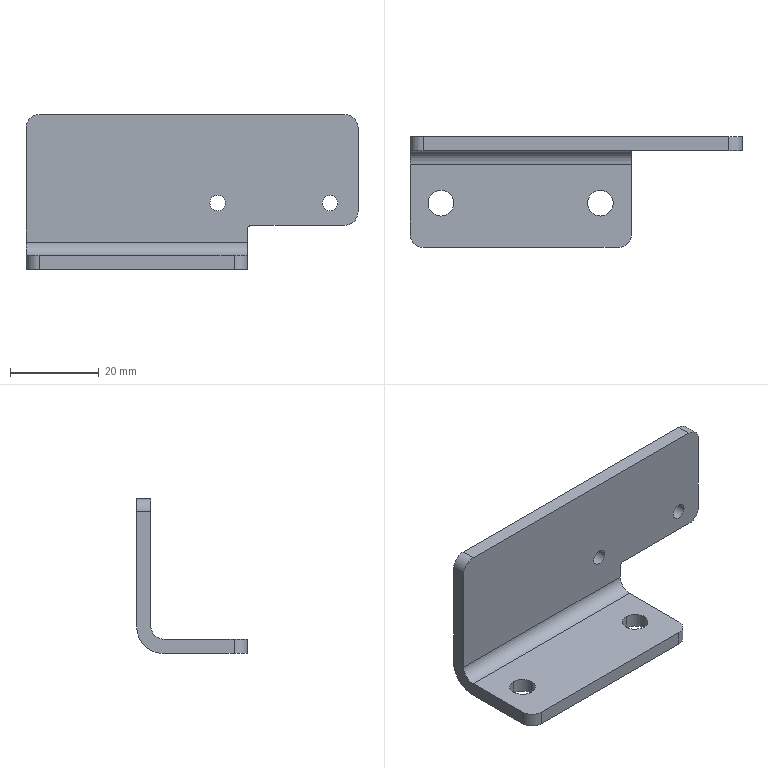Part | STEP file | J014-EBZ05-02-06-Part-1 | 1 solid | 26 faces | box 75 x 25 x 35 mm | volume 10537 mm3 | cylinder 16 | plane 10 | commonest cylinder face diameters 6 x6 3.5 x4 5.8 x4 2 x1 12 x1
STEP:
#1=CARTESIAN_POINT('',(41.55,0.,15.));
#2=VERTEX_POINT('',#1);
#3=CARTESIAN_POINT('',(45.05,0.,15.));
#4=VERTEX_POINT('',#3);
#5=CARTESIAN_POINT('',(43.3,0.,15.));
#6=DIRECTION('',(0.,-1.,0.));
#7=DIRECTION('',(1.,0.,0.));
#8=AXIS2_PLACEMENT_3D('',#5,#6,#7);
#9=CIRCLE('',#8,1.75);
#10=EDGE_CURVE('',#2,#4,#9,.T.);
#11=ORIENTED_EDGE('',*,*,#10,.F.);
#12=CARTESIAN_POINT('',(41.55,-3.2,15.));
#13=VERTEX_POINT('',#12);
#14=CARTESIAN_POINT('',(41.55,0.,15.));
#15=DIRECTION('',(0.,-1.,0.));
#16=VECTOR('',#15,1000.);
#17=LINE('',#14,#16);
#18=EDGE_CURVE('',#2,#13,#17,.T.);
#19=ORIENTED_EDGE('',*,*,#18,.T.);
#20=CARTESIAN_POINT('',(45.05,-3.2,15.));
#21=VERTEX_POINT('',#20);
#22=CARTESIAN_POINT('',(43.3,-3.2,15.));
#23=DIRECTION('',(0.,1.,0.));
#24=DIRECTION('',(-1.,0.,0.));
#25=AXIS2_PLACEMENT_3D('',#22,#23,#24);
#26=CIRCLE('',#25,1.75);
#27=EDGE_CURVE('',#21,#13,#26,.T.);
#28=ORIENTED_EDGE('',*,*,#27,.F.);
#29=CARTESIAN_POINT('',(45.05,0.,15.));
#30=DIRECTION('',(0.,-1.,0.));
#31=VECTOR('',#30,1000.);
#32=LINE('',#29,#31);
#33=EDGE_CURVE('',#4,#21,#32,.T.);
#34=ORIENTED_EDGE('',*,*,#33,.F.);
#35=EDGE_LOOP('',(#11,#19,#28,#34));
#36=FACE_OUTER_BOUND('',#35,.T.);
#37=CARTESIAN_POINT('',(43.3,0.,15.));
#38=DIRECTION('',(0.,-1.,0.));
#39=DIRECTION('',(1.,0.,0.));
#40=AXIS2_PLACEMENT_3D('',#37,#38,#39);
#41=CYLINDRICAL_SURFACE('',#40,1.75);
#42=ADVANCED_FACE('',(#36),#41,.F.);
#43=CARTESIAN_POINT('',(66.95,0.,15.));
#44=VERTEX_POINT('',#43);
#45=CARTESIAN_POINT('',(70.45,0.,15.));
#46=VERTEX_POINT('',#45);
#47=CARTESIAN_POINT('',(68.7,0.,15.));
#48=DIRECTION('',(0.,-1.,0.));
#49=DIRECTION('',(1.,0.,0.));
#50=AXIS2_PLACEMENT_3D('',#47,#48,#49);
#51=CIRCLE('',#50,1.75);
#52=EDGE_CURVE('',#44,#46,#51,.T.);
#53=ORIENTED_EDGE('',*,*,#52,.F.);
#54=CARTESIAN_POINT('',(66.95,-3.2,15.));
#55=VERTEX_POINT('',#54);
#56=CARTESIAN_POINT('',(66.95,0.,15.));
#57=DIRECTION('',(0.,-1.,0.));
#58=VECTOR('',#57,1000.);
#59=LINE('',#56,#58);
#60=EDGE_CURVE('',#44,#55,#59,.T.);
#61=ORIENTED_EDGE('',*,*,#60,.T.);
#62=CARTESIAN_POINT('',(70.45,-3.2,15.));
#63=VERTEX_POINT('',#62);
#64=CARTESIAN_POINT('',(68.7,-3.2,15.));
#65=DIRECTION('',(0.,1.,0.));
#66=DIRECTION('',(-1.,0.,0.));
#67=AXIS2_PLACEMENT_3D('',#64,#65,#66);
#68=CIRCLE('',#67,1.75);
#69=EDGE_CURVE('',#63,#55,#68,.T.);
#70=ORIENTED_EDGE('',*,*,#69,.F.);
#71=CARTESIAN_POINT('',(70.45,0.,15.));
#72=DIRECTION('',(0.,-1.,0.));
#73=VECTOR('',#72,1000.);
#74=LINE('',#71,#73);
#75=EDGE_CURVE('',#46,#63,#74,.T.);
#76=ORIENTED_EDGE('',*,*,#75,.F.);
#77=EDGE_LOOP('',(#53,#61,#70,#76));
#78=FACE_OUTER_BOUND('',#77,.T.);
#79=CARTESIAN_POINT('',(68.7,0.,15.));
#80=DIRECTION('',(0.,-1.,0.));
#81=DIRECTION('',(1.,0.,0.));
#82=AXIS2_PLACEMENT_3D('',#79,#80,#81);
#83=CYLINDRICAL_SURFACE('',#82,1.75);
#84=ADVANCED_FACE('',(#78),#83,.F.);
#85=CARTESIAN_POINT('',(7.,-17.9,3.2));
#86=VERTEX_POINT('',#85);
#87=CARTESIAN_POINT('',(7.,-12.1,3.2));
#88=VERTEX_POINT('',#87);
#89=CARTESIAN_POINT('',(7.,-15.,3.2));
#90=DIRECTION('',(0.,0.,-1.));
#91=DIRECTION('',(0.,1.,0.));
#92=AXIS2_PLACEMENT_3D('',#89,#90,#91);
#93=CIRCLE('',#92,2.9);
#94=EDGE_CURVE('',#86,#88,#93,.T.);
#95=ORIENTED_EDGE('',*,*,#94,.F.);
#96=CARTESIAN_POINT('',(7.,-17.9,0.));
#97=VERTEX_POINT('',#96);
#98=CARTESIAN_POINT('',(7.,-17.9,3.2));
#99=DIRECTION('',(0.,0.,-1.));
#100=VECTOR('',#99,1000.);
#101=LINE('',#98,#100);
#102=EDGE_CURVE('',#86,#97,#101,.T.);
#103=ORIENTED_EDGE('',*,*,#102,.T.);
#104=CARTESIAN_POINT('',(7.,-12.1,0.));
#105=VERTEX_POINT('',#104);
#106=CARTESIAN_POINT('',(7.,-15.,0.));
#107=DIRECTION('',(0.,0.,-1.));
#108=DIRECTION('',(0.,1.,0.));
#109=AXIS2_PLACEMENT_3D('',#106,#107,#108);
#110=CIRCLE('',#109,2.9);
#111=EDGE_CURVE('',#97,#105,#110,.T.);
#112=ORIENTED_EDGE('',*,*,#111,.T.);
#113=CARTESIAN_POINT('',(7.,-12.1,3.2));
#114=DIRECTION('',(0.,0.,-1.));
#115=VECTOR('',#114,1000.);
#116=LINE('',#113,#115);
#117=EDGE_CURVE('',#88,#105,#116,.T.);
#118=ORIENTED_EDGE('',*,*,#117,.F.);
#119=EDGE_LOOP('',(#95,#103,#112,#118));
#120=FACE_OUTER_BOUND('',#119,.T.);
#121=CARTESIAN_POINT('',(7.,-15.,3.2));
#122=DIRECTION('',(0.,0.,-1.));
#123=DIRECTION('',(0.,1.,0.));
#124=AXIS2_PLACEMENT_3D('',#121,#122,#123);
#125=CYLINDRICAL_SURFACE('',#124,2.9);
#126=ADVANCED_FACE('',(#120),#125,.F.);
#127=CARTESIAN_POINT('',(43.,-17.9,3.2));
#128=VERTEX_POINT('',#127);
#129=CARTESIAN_POINT('',(43.,-12.1,3.2));
#130=VERTEX_POINT('',#129);
#131=CARTESIAN_POINT('',(43.,-15.,3.2));
#132=DIRECTION('',(0.,0.,-1.));
#133=DIRECTION('',(0.,1.,0.));
#134=AXIS2_PLACEMENT_3D('',#131,#132,#133);
#135=CIRCLE('',#134,2.9);
#136=EDGE_CURVE('',#128,#130,#135,.T.);
#137=ORIENTED_EDGE('',*,*,#136,.F.);
#138=CARTESIAN_POINT('',(43.,-17.9,0.));
#139=VERTEX_POINT('',#138);
#140=CARTESIAN_POINT('',(43.,-17.9,3.2));
#141=DIRECTION('',(0.,0.,-1.));
#142=VECTOR('',#141,1000.);
#143=LINE('',#140,#142);
#144=EDGE_CURVE('',#128,#139,#143,.T.);
#145=ORIENTED_EDGE('',*,*,#144,.T.);
#146=CARTESIAN_POINT('',(43.,-12.1,0.));
#147=VERTEX_POINT('',#146);
#148=CARTESIAN_POINT('',(43.,-15.,0.));
#149=DIRECTION('',(0.,0.,-1.));
#150=DIRECTION('',(0.,1.,0.));
#151=AXIS2_PLACEMENT_3D('',#148,#149,#150);
#152=CIRCLE('',#151,2.9);
#153=EDGE_CURVE('',#139,#147,#152,.T.);
#154=ORIENTED_EDGE('',*,*,#153,.T.);
#155=CARTESIAN_POINT('',(43.,-12.1,3.2));
#156=DIRECTION('',(0.,0.,-1.));
#157=VECTOR('',#156,1000.);
#158=LINE('',#155,#157);
#159=EDGE_CURVE('',#130,#147,#158,.T.);
#160=ORIENTED_EDGE('',*,*,#159,.F.);
#161=EDGE_LOOP('',(#137,#145,#154,#160));
#162=FACE_OUTER_BOUND('',#161,.T.);
#163=CARTESIAN_POINT('',(43.,-15.,3.2));
#164=DIRECTION('',(0.,0.,-1.));
#165=DIRECTION('',(0.,1.,0.));
#166=AXIS2_PLACEMENT_3D('',#163,#164,#165);
#167=CYLINDRICAL_SURFACE('',#166,2.9);
#168=ADVANCED_FACE('',(#162),#167,.F.);
#169=CARTESIAN_POINT('',(7.,-15.,3.2));
#170=DIRECTION('',(0.,0.,-1.));
#171=DIRECTION('',(0.,1.,0.));
#172=AXIS2_PLACEMENT_3D('',#169,#170,#171);
#173=CIRCLE('',#172,2.9);
#174=EDGE_CURVE('',#88,#86,#173,.T.);
#175=ORIENTED_EDGE('',*,*,#174,.T.);
#176=ORIENTED_EDGE('',*,*,#94,.T.);
#177=EDGE_LOOP('',(#175,#176));
#178=FACE_BOUND('',#177,.T.);
#179=CARTESIAN_POINT('',(43.,-15.,3.2));
#180=DIRECTION('',(0.,0.,-1.));
#181=DIRECTION('',(0.,1.,0.));
#182=AXIS2_PLACEMENT_3D('',#179,#180,#181);
#183=CIRCLE('',#182,2.9);
#184=EDGE_CURVE('',#130,#128,#183,.T.);
#185=ORIENTED_EDGE('',*,*,#184,.T.);
#186=ORIENTED_EDGE('',*,*,#136,.T.);
#187=EDGE_LOOP('',(#185,#186));
#188=FACE_BOUND('',#187,.T.);
#189=CARTESIAN_POINT('',(47.,-25.,3.2));
#190=VERTEX_POINT('',#189);
#191=CARTESIAN_POINT('',(3.,-25.,3.2));
#192=VERTEX_POINT('',#191);
#193=CARTESIAN_POINT('',(25.,-25.,3.2));
#194=DIRECTION('',(-1.,0.,0.));
#195=VECTOR('',#194,1000.);
#196=LINE('',#193,#195);
#197=EDGE_CURVE('',#190,#192,#196,.T.);
#198=ORIENTED_EDGE('',*,*,#197,.F.);
#199=CARTESIAN_POINT('',(50.,-22.,3.2));
#200=VERTEX_POINT('',#199);
#201=CARTESIAN_POINT('',(47.,-22.,3.2));
#202=DIRECTION('',(0.,0.,1.));
#203=DIRECTION('',(0.,-1.,0.));
#204=AXIS2_PLACEMENT_3D('',#201,#202,#203);
#205=CIRCLE('',#204,3.);
#206=EDGE_CURVE('',#190,#200,#205,.T.);
#207=ORIENTED_EDGE('',*,*,#206,.T.);
#208=CARTESIAN_POINT('',(50.,-6.2,3.2));
#209=VERTEX_POINT('',#208);
#210=CARTESIAN_POINT('',(50.,-12.5,3.2));
#211=DIRECTION('',(0.,-1.,0.));
#212=VECTOR('',#211,1000.);
#213=LINE('',#210,#212);
#214=EDGE_CURVE('',#209,#200,#213,.T.);
#215=ORIENTED_EDGE('',*,*,#214,.F.);
#216=CARTESIAN_POINT('',(0.,-6.2,3.2));
#217=VERTEX_POINT('',#216);
#218=CARTESIAN_POINT('',(0.,-6.2,3.2));
#219=DIRECTION('',(-1.,0.,0.));
#220=VECTOR('',#219,1000.);
#221=LINE('',#218,#220);
#222=EDGE_CURVE('',#209,#217,#221,.T.);
#223=ORIENTED_EDGE('',*,*,#222,.T.);
#224=CARTESIAN_POINT('',(0.,-22.,3.2));
#225=VERTEX_POINT('',#224);
#226=CARTESIAN_POINT('',(0.,-12.5,3.2));
#227=DIRECTION('',(0.,1.,0.));
#228=VECTOR('',#227,1000.);
#229=LINE('',#226,#228);
#230=EDGE_CURVE('',#225,#217,#229,.T.);
#231=ORIENTED_EDGE('',*,*,#230,.F.);
#232=CARTESIAN_POINT('',(3.,-22.,3.2));
#233=DIRECTION('',(0.,0.,1.));
#234=DIRECTION('',(0.,-1.,0.));
#235=AXIS2_PLACEMENT_3D('',#232,#233,#234);
#236=CIRCLE('',#235,3.);
#237=EDGE_CURVE('',#225,#192,#236,.T.);
#238=ORIENTED_EDGE('',*,*,#237,.T.);
#239=EDGE_LOOP('',(#198,#207,#215,#223,#231,#238));
#240=FACE_OUTER_BOUND('',#239,.T.);
#241=CARTESIAN_POINT('',(25.,-12.5,3.2));
#242=DIRECTION('',(0.,0.,1.));
#243=DIRECTION('',(0.,-1.,0.));
#244=AXIS2_PLACEMENT_3D('',#241,#242,#243);
#245=PLANE('',#244);
#246=ADVANCED_FACE('',(#178,#188,#240),#245,.T.);
#247=CARTESIAN_POINT('',(0.,-3.2,6.2));
#248=VERTEX_POINT('',#247);
#249=CARTESIAN_POINT('',(0.,-3.2,32.));
#250=VERTEX_POINT('',#249);
#251=CARTESIAN_POINT('',(0.,-3.2,3.2));
#252=DIRECTION('',(0.,0.,1.));
#253=VECTOR('',#252,1000.);
#254=LINE('',#251,#253);
#255=EDGE_CURVE('',#248,#250,#254,.T.);
#256=ORIENTED_EDGE('',*,*,#255,.T.);
#257=CARTESIAN_POINT('',(0.,0.,32.));
#258=VERTEX_POINT('',#257);
#259=CARTESIAN_POINT('',(0.,-12.5,32.));
#260=DIRECTION('',(0.,1.,0.));
#261=VECTOR('',#260,1000.);
#262=LINE('',#259,#261);
#263=EDGE_CURVE('',#250,#258,#262,.T.);
#264=ORIENTED_EDGE('',*,*,#263,.T.);
#265=CARTESIAN_POINT('',(0.,0.,6.));
#266=VERTEX_POINT('',#265);
#267=CARTESIAN_POINT('',(0.,0.,0.));
#268=DIRECTION('',(0.,0.,1.));
#269=VECTOR('',#268,1000.);
#270=LINE('',#267,#269);
#271=EDGE_CURVE('',#266,#258,#270,.T.);
#272=ORIENTED_EDGE('',*,*,#271,.F.);
#273=CARTESIAN_POINT('',(0.,-6.,0.));
#274=VERTEX_POINT('',#273);
#275=CARTESIAN_POINT('',(0.,-6.,6.));
#276=DIRECTION('',(-1.,0.,0.));
#277=DIRECTION('',(0.,0.,-1.));
#278=AXIS2_PLACEMENT_3D('',#275,#276,#277);
#279=CIRCLE('',#278,6.);
#280=EDGE_CURVE('',#266,#274,#279,.T.);
#281=ORIENTED_EDGE('',*,*,#280,.T.);
#282=CARTESIAN_POINT('',(0.,-22.,0.));
#283=VERTEX_POINT('',#282);
#284=CARTESIAN_POINT('',(0.,-12.5,0.));
#285=DIRECTION('',(0.,-1.,0.));
#286=VECTOR('',#285,1000.);
#287=LINE('',#284,#286);
#288=EDGE_CURVE('',#274,#283,#287,.T.);
#289=ORIENTED_EDGE('',*,*,#288,.T.);
#290=CARTESIAN_POINT('',(0.,-22.,0.));
#291=DIRECTION('',(0.,0.,1.));
#292=VECTOR('',#291,1000.);
#293=LINE('',#290,#292);
#294=EDGE_CURVE('',#283,#225,#293,.T.);
#295=ORIENTED_EDGE('',*,*,#294,.T.);
#296=ORIENTED_EDGE('',*,*,#230,.T.);
#297=CARTESIAN_POINT('',(0.,-6.2,6.2));
#298=DIRECTION('',(1.,0.,0.));
#299=DIRECTION('',(0.,0.,-1.));
#300=AXIS2_PLACEMENT_3D('',#297,#298,#299);
#301=CIRCLE('',#300,3.);
#302=EDGE_CURVE('',#217,#248,#301,.T.);
#303=ORIENTED_EDGE('',*,*,#302,.T.);
#304=EDGE_LOOP('',(#256,#264,#272,#281,#289,#295,#296,#303));
#305=FACE_OUTER_BOUND('',#304,.T.);
#306=CARTESIAN_POINT('',(0.,-12.5,0.));
#307=DIRECTION('',(-1.,0.,0.));
#308=DIRECTION('',(0.,0.,-1.));
#309=AXIS2_PLACEMENT_3D('',#306,#307,#308);
#310=PLANE('',#309);
#311=ADVANCED_FACE('',(#305),#310,.T.);
#312=CARTESIAN_POINT('',(43.3,0.,15.));
#313=DIRECTION('',(0.,-1.,0.));
#314=DIRECTION('',(1.,0.,0.));
#315=AXIS2_PLACEMENT_3D('',#312,#313,#314);
#316=CIRCLE('',#315,1.75);
#317=EDGE_CURVE('',#4,#2,#316,.T.);
#318=ORIENTED_EDGE('',*,*,#317,.T.);
#319=ORIENTED_EDGE('',*,*,#10,.T.);
#320=EDGE_LOOP('',(#318,#319));
#321=FACE_BOUND('',#320,.T.);
#322=CARTESIAN_POINT('',(68.7,0.,15.));
#323=DIRECTION('',(0.,-1.,0.));
#324=DIRECTION('',(1.,0.,0.));
#325=AXIS2_PLACEMENT_3D('',#322,#323,#324);
#326=CIRCLE('',#325,1.75);
#327=EDGE_CURVE('',#46,#44,#326,.T.);
#328=ORIENTED_EDGE('',*,*,#327,.T.);
#329=ORIENTED_EDGE('',*,*,#52,.T.);
#330=EDGE_LOOP('',(#328,#329));
#331=FACE_BOUND('',#330,.T.);
#332=CARTESIAN_POINT('',(75.,0.,13.));
#333=VERTEX_POINT('',#332);
#334=CARTESIAN_POINT('',(75.,0.,32.));
#335=VERTEX_POINT('',#334);
#336=CARTESIAN_POINT('',(75.,0.,22.5));
#337=DIRECTION('',(0.,0.,1.));
#338=VECTOR('',#337,1000.);
#339=LINE('',#336,#338);
#340=EDGE_CURVE('',#333,#335,#339,.T.);
#341=ORIENTED_EDGE('',*,*,#340,.F.);
#342=CARTESIAN_POINT('',(72.,0.,10.));
#343=VERTEX_POINT('',#342);
#344=CARTESIAN_POINT('',(72.,0.,13.));
#345=DIRECTION('',(0.,1.,0.));
#346=DIRECTION('',(0.,0.,1.));
#347=AXIS2_PLACEMENT_3D('',#344,#345,#346);
#348=CIRCLE('',#347,3.);
#349=EDGE_CURVE('',#333,#343,#348,.T.);
#350=ORIENTED_EDGE('',*,*,#349,.T.);
#351=CARTESIAN_POINT('',(51.,0.,10.));
#352=VERTEX_POINT('',#351);
#353=CARTESIAN_POINT('',(62.5,0.,10.));
#354=DIRECTION('',(1.,0.,0.));
#355=VECTOR('',#354,1000.);
#356=LINE('',#353,#355);
#357=EDGE_CURVE('',#352,#343,#356,.T.);
#358=ORIENTED_EDGE('',*,*,#357,.F.);
#359=CARTESIAN_POINT('',(50.,0.,9.));
#360=VERTEX_POINT('',#359);
#361=CARTESIAN_POINT('',(51.,0.,9.));
#362=DIRECTION('',(0.,-1.,0.));
#363=DIRECTION('',(0.,0.,1.));
#364=AXIS2_PLACEMENT_3D('',#361,#362,#363);
#365=CIRCLE('',#364,1.);
#366=EDGE_CURVE('',#352,#360,#365,.T.);
#367=ORIENTED_EDGE('',*,*,#366,.T.);
#368=CARTESIAN_POINT('',(50.,0.,6.));
#369=VERTEX_POINT('',#368);
#370=CARTESIAN_POINT('',(50.,0.,0.));
#371=DIRECTION('',(0.,0.,1.));
#372=VECTOR('',#371,1000.);
#373=LINE('',#370,#372);
#374=EDGE_CURVE('',#369,#360,#373,.T.);
#375=ORIENTED_EDGE('',*,*,#374,.F.);
#376=CARTESIAN_POINT('',(25.,0.,6.));
#377=DIRECTION('',(-1.,0.,0.));
#378=VECTOR('',#377,1000.);
#379=LINE('',#376,#378);
#380=EDGE_CURVE('',#369,#266,#379,.T.);
#381=ORIENTED_EDGE('',*,*,#380,.T.);
#382=ORIENTED_EDGE('',*,*,#271,.T.);
#383=CARTESIAN_POINT('',(3.,0.,35.));
#384=VERTEX_POINT('',#383);
#385=CARTESIAN_POINT('',(3.,0.,32.));
#386=DIRECTION('',(0.,1.,0.));
#387=DIRECTION('',(0.,0.,1.));
#388=AXIS2_PLACEMENT_3D('',#385,#386,#387);
#389=CIRCLE('',#388,3.);
#390=EDGE_CURVE('',#258,#384,#389,.T.);
#391=ORIENTED_EDGE('',*,*,#390,.T.);
#392=CARTESIAN_POINT('',(72.,0.,35.));
#393=VERTEX_POINT('',#392);
#394=CARTESIAN_POINT('',(25.,0.,35.));
#395=DIRECTION('',(1.,0.,0.));
#396=VECTOR('',#395,1000.);
#397=LINE('',#394,#396);
#398=EDGE_CURVE('',#384,#393,#397,.T.);
#399=ORIENTED_EDGE('',*,*,#398,.T.);
#400=CARTESIAN_POINT('',(72.,0.,32.));
#401=DIRECTION('',(0.,1.,0.));
#402=DIRECTION('',(0.,0.,1.));
#403=AXIS2_PLACEMENT_3D('',#400,#401,#402);
#404=CIRCLE('',#403,3.);
#405=EDGE_CURVE('',#393,#335,#404,.T.);
#406=ORIENTED_EDGE('',*,*,#405,.T.);
#407=EDGE_LOOP('',(#341,#350,#358,#367,#375,#381,#382,#391,#399,#406));
#408=FACE_OUTER_BOUND('',#407,.T.);
#409=CARTESIAN_POINT('',(25.,0.,0.));
#410=DIRECTION('',(0.,1.,0.));
#411=DIRECTION('',(0.,0.,1.));
#412=AXIS2_PLACEMENT_3D('',#409,#410,#411);
#413=PLANE('',#412);
#414=ADVANCED_FACE('',(#321,#331,#408),#413,.T.);
#415=ORIENTED_EDGE('',*,*,#374,.T.);
#416=CARTESIAN_POINT('',(50.,-3.2,9.));
#417=VERTEX_POINT('',#416);
#418=CARTESIAN_POINT('',(50.,-3.2,9.));
#419=DIRECTION('',(0.,-1.,0.));
#420=VECTOR('',#419,1000.);
#421=LINE('',#418,#420);
#422=EDGE_CURVE('',#360,#417,#421,.T.);
#423=ORIENTED_EDGE('',*,*,#422,.T.);
#424=CARTESIAN_POINT('',(50.,-3.2,6.2));
#425=VERTEX_POINT('',#424);
#426=CARTESIAN_POINT('',(50.,-3.2,3.2));
#427=DIRECTION('',(0.,0.,1.));
#428=VECTOR('',#427,1000.);
#429=LINE('',#426,#428);
#430=EDGE_CURVE('',#425,#417,#429,.T.);
#431=ORIENTED_EDGE('',*,*,#430,.F.);
#432=CARTESIAN_POINT('',(50.,-6.2,6.2));
#433=DIRECTION('',(-1.,0.,0.));
#434=DIRECTION('',(0.,0.,1.));
#435=AXIS2_PLACEMENT_3D('',#432,#433,#434);
#436=CIRCLE('',#435,3.);
#437=EDGE_CURVE('',#425,#209,#436,.T.);
#438=ORIENTED_EDGE('',*,*,#437,.T.);
#439=ORIENTED_EDGE('',*,*,#214,.T.);
#440=CARTESIAN_POINT('',(50.,-22.,0.));
#441=VERTEX_POINT('',#440);
#442=CARTESIAN_POINT('',(50.,-22.,0.));
#443=DIRECTION('',(0.,0.,-1.));
#444=VECTOR('',#443,1000.);
#445=LINE('',#442,#444);
#446=EDGE_CURVE('',#200,#441,#445,.T.);
#447=ORIENTED_EDGE('',*,*,#446,.T.);
#448=CARTESIAN_POINT('',(50.,-6.,0.));
#449=VERTEX_POINT('',#448);
#450=CARTESIAN_POINT('',(50.,-12.5,0.));
#451=DIRECTION('',(0.,1.,0.));
#452=VECTOR('',#451,1000.);
#453=LINE('',#450,#452);
#454=EDGE_CURVE('',#441,#449,#453,.T.);
#455=ORIENTED_EDGE('',*,*,#454,.T.);
#456=CARTESIAN_POINT('',(50.,-6.,6.));
#457=DIRECTION('',(1.,0.,0.));
#458=DIRECTION('',(0.,0.,1.));
#459=AXIS2_PLACEMENT_3D('',#456,#457,#458);
#460=CIRCLE('',#459,6.);
#461=EDGE_CURVE('',#449,#369,#460,.T.);
#462=ORIENTED_EDGE('',*,*,#461,.T.);
#463=EDGE_LOOP('',(#415,#423,#431,#438,#439,#447,#455,#462));
#464=FACE_OUTER_BOUND('',#463,.T.);
#465=CARTESIAN_POINT('',(50.,-12.5,0.));
#466=DIRECTION('',(1.,0.,0.));
#467=DIRECTION('',(0.,0.,1.));
#468=AXIS2_PLACEMENT_3D('',#465,#466,#467);
#469=PLANE('',#468);
#470=ADVANCED_FACE('',(#464),#469,.T.);
#471=CARTESIAN_POINT('',(7.,-15.,0.));
#472=DIRECTION('',(0.,0.,-1.));
#473=DIRECTION('',(0.,1.,0.));
#474=AXIS2_PLACEMENT_3D('',#471,#472,#473);
#475=CIRCLE('',#474,2.9);
#476=EDGE_CURVE('',#105,#97,#475,.T.);
#477=ORIENTED_EDGE('',*,*,#476,.F.);
#478=ORIENTED_EDGE('',*,*,#111,.F.);
#479=EDGE_LOOP('',(#477,#478));
#480=FACE_BOUND('',#479,.T.);
#481=CARTESIAN_POINT('',(43.,-15.,0.));
#482=DIRECTION('',(0.,0.,-1.));
#483=DIRECTION('',(0.,1.,0.));
#484=AXIS2_PLACEMENT_3D('',#481,#482,#483);
#485=CIRCLE('',#484,2.9);
#486=EDGE_CURVE('',#147,#139,#485,.T.);
#487=ORIENTED_EDGE('',*,*,#486,.F.);
#488=ORIENTED_EDGE('',*,*,#153,.F.);
#489=EDGE_LOOP('',(#487,#488));
#490=FACE_BOUND('',#489,.T.);
#491=ORIENTED_EDGE('',*,*,#454,.F.);
#492=CARTESIAN_POINT('',(47.,-25.,0.));
#493=VERTEX_POINT('',#492);
#494=CARTESIAN_POINT('',(47.,-22.,0.));
#495=DIRECTION('',(0.,0.,-1.));
#496=DIRECTION('',(0.,1.,0.));
#497=AXIS2_PLACEMENT_3D('',#494,#495,#496);
#498=CIRCLE('',#497,3.);
#499=EDGE_CURVE('',#441,#493,#498,.T.);
#500=ORIENTED_EDGE('',*,*,#499,.T.);
#501=CARTESIAN_POINT('',(3.,-25.,0.));
#502=VERTEX_POINT('',#501);
#503=CARTESIAN_POINT('',(25.,-25.,0.));
#504=DIRECTION('',(1.,0.,0.));
#505=VECTOR('',#504,1000.);
#506=LINE('',#503,#505);
#507=EDGE_CURVE('',#502,#493,#506,.T.);
#508=ORIENTED_EDGE('',*,*,#507,.F.);
#509=CARTESIAN_POINT('',(3.,-22.,0.));
#510=DIRECTION('',(0.,0.,-1.));
#511=DIRECTION('',(0.,1.,0.));
#512=AXIS2_PLACEMENT_3D('',#509,#510,#511);
#513=CIRCLE('',#512,3.);
#514=EDGE_CURVE('',#502,#283,#513,.T.);
#515=ORIENTED_EDGE('',*,*,#514,.T.);
#516=ORIENTED_EDGE('',*,*,#288,.F.);
#517=CARTESIAN_POINT('',(25.,-6.,0.));
#518=DIRECTION('',(1.,0.,0.));
#519=VECTOR('',#518,1000.);
#520=LINE('',#517,#519);
#521=EDGE_CURVE('',#274,#449,#520,.T.);
#522=ORIENTED_EDGE('',*,*,#521,.T.);
#523=EDGE_LOOP('',(#491,#500,#508,#515,#516,#522));
#524=FACE_OUTER_BOUND('',#523,.T.);
#525=CARTESIAN_POINT('',(25.,-12.5,0.));
#526=DIRECTION('',(0.,0.,-1.));
#527=DIRECTION('',(0.,1.,0.));
#528=AXIS2_PLACEMENT_3D('',#525,#526,#527);
#529=PLANE('',#528);
#530=ADVANCED_FACE('',(#480,#490,#524),#529,.T.);
#531=ORIENTED_EDGE('',*,*,#507,.T.);
#532=CARTESIAN_POINT('',(47.,-25.,0.));
#533=DIRECTION('',(0.,0.,1.));
#534=VECTOR('',#533,1000.);
#535=LINE('',#532,#534);
#536=EDGE_CURVE('',#493,#190,#535,.T.);
#537=ORIENTED_EDGE('',*,*,#536,.T.);
#538=ORIENTED_EDGE('',*,*,#197,.T.);
#539=CARTESIAN_POINT('',(3.,-25.,0.));
#540=DIRECTION('',(0.,0.,-1.));
#541=VECTOR('',#540,1000.);
#542=LINE('',#539,#541);
#543=EDGE_CURVE('',#192,#502,#542,.T.);
#544=ORIENTED_EDGE('',*,*,#543,.T.);
#545=EDGE_LOOP('',(#531,#537,#538,#544));
#546=FACE_OUTER_BOUND('',#545,.T.);
#547=CARTESIAN_POINT('',(25.,-25.,0.));
#548=DIRECTION('',(0.,-1.,0.));
#549=DIRECTION('',(0.,0.,-1.));
#550=AXIS2_PLACEMENT_3D('',#547,#548,#549);
#551=PLANE('',#550);
#552=ADVANCED_FACE('',(#546),#551,.T.);
#553=CARTESIAN_POINT('',(72.,-3.2,35.));
#554=VERTEX_POINT('',#553);
#555=CARTESIAN_POINT('',(3.,-3.2,35.));
#556=VERTEX_POINT('',#555);
#557=CARTESIAN_POINT('',(25.,-3.2,35.));
#558=DIRECTION('',(-1.,0.,0.));
#559=VECTOR('',#558,1000.);
#560=LINE('',#557,#559);
#561=EDGE_CURVE('',#554,#556,#560,.T.);
#562=ORIENTED_EDGE('',*,*,#561,.F.);
#563=CARTESIAN_POINT('',(72.,-1.6,35.));
#564=DIRECTION('',(0.,1.,0.));
#565=VECTOR('',#564,1000.);
#566=LINE('',#563,#565);
#567=EDGE_CURVE('',#554,#393,#566,.T.);
#568=ORIENTED_EDGE('',*,*,#567,.T.);
#569=ORIENTED_EDGE('',*,*,#398,.F.);
#570=CARTESIAN_POINT('',(3.,-1.6,35.));
#571=DIRECTION('',(0.,-1.,0.));
#572=VECTOR('',#571,1000.);
#573=LINE('',#570,#572);
#574=EDGE_CURVE('',#384,#556,#573,.T.);
#575=ORIENTED_EDGE('',*,*,#574,.T.);
#576=EDGE_LOOP('',(#562,#568,#569,#575));
#577=FACE_OUTER_BOUND('',#576,.T.);
#578=CARTESIAN_POINT('',(25.,-1.6,35.));
#579=DIRECTION('',(0.,0.,1.));
#580=DIRECTION('',(0.,1.,0.));
#581=AXIS2_PLACEMENT_3D('',#578,#579,#580);
#582=PLANE('',#581);
#583=ADVANCED_FACE('',(#577),#582,.T.);
#584=ORIENTED_EDGE('',*,*,#27,.T.);
#585=CARTESIAN_POINT('',(43.3,-3.2,15.));
#586=DIRECTION('',(0.,1.,0.));
#587=DIRECTION('',(-1.,0.,0.));
#588=AXIS2_PLACEMENT_3D('',#585,#586,#587);
#589=CIRCLE('',#588,1.75);
#590=EDGE_CURVE('',#13,#21,#589,.T.);
#591=ORIENTED_EDGE('',*,*,#590,.T.);
#592=EDGE_LOOP('',(#584,#591));
#593=FACE_BOUND('',#592,.T.);
#594=ORIENTED_EDGE('',*,*,#69,.T.);
#595=CARTESIAN_POINT('',(68.7,-3.2,15.));
#596=DIRECTION('',(0.,1.,0.));
#597=DIRECTION('',(-1.,0.,0.));
#598=AXIS2_PLACEMENT_3D('',#595,#596,#597);
#599=CIRCLE('',#598,1.75);
#600=EDGE_CURVE('',#55,#63,#599,.T.);
#601=ORIENTED_EDGE('',*,*,#600,.T.);
#602=EDGE_LOOP('',(#594,#601));
#603=FACE_BOUND('',#602,.T.);
#604=CARTESIAN_POINT('',(72.,-3.2,10.));
#605=VERTEX_POINT('',#604);
#606=CARTESIAN_POINT('',(51.,-3.2,10.));
#607=VERTEX_POINT('',#606);
#608=CARTESIAN_POINT('',(62.5,-3.2,10.));
#609=DIRECTION('',(-1.,0.,0.));
#610=VECTOR('',#609,1000.);
#611=LINE('',#608,#610);
#612=EDGE_CURVE('',#605,#607,#611,.T.);
#613=ORIENTED_EDGE('',*,*,#612,.F.);
#614=CARTESIAN_POINT('',(75.,-3.2,13.));
#615=VERTEX_POINT('',#614);
#616=CARTESIAN_POINT('',(72.,-3.2,13.));
#617=DIRECTION('',(0.,-1.,0.));
#618=DIRECTION('',(0.,0.,-1.));
#619=AXIS2_PLACEMENT_3D('',#616,#617,#618);
#620=CIRCLE('',#619,3.);
#621=EDGE_CURVE('',#605,#615,#620,.T.);
#622=ORIENTED_EDGE('',*,*,#621,.T.);
#623=CARTESIAN_POINT('',(75.,-3.2,32.));
#624=VERTEX_POINT('',#623);
#625=CARTESIAN_POINT('',(75.,-3.2,22.5));
#626=DIRECTION('',(0.,0.,-1.));
#627=VECTOR('',#626,1000.);
#628=LINE('',#625,#627);
#629=EDGE_CURVE('',#624,#615,#628,.T.);
#630=ORIENTED_EDGE('',*,*,#629,.F.);
#631=CARTESIAN_POINT('',(72.,-3.2,32.));
#632=DIRECTION('',(0.,-1.,0.));
#633=DIRECTION('',(0.,0.,-1.));
#634=AXIS2_PLACEMENT_3D('',#631,#632,#633);
#635=CIRCLE('',#634,3.);
#636=EDGE_CURVE('',#624,#554,#635,.T.);
#637=ORIENTED_EDGE('',*,*,#636,.T.);
#638=ORIENTED_EDGE('',*,*,#561,.T.);
#639=CARTESIAN_POINT('',(3.,-3.2,32.));
#640=DIRECTION('',(0.,-1.,0.));
#641=DIRECTION('',(0.,0.,-1.));
#642=AXIS2_PLACEMENT_3D('',#639,#640,#641);
#643=CIRCLE('',#642,3.);
#644=EDGE_CURVE('',#556,#250,#643,.T.);
#645=ORIENTED_EDGE('',*,*,#644,.T.);
#646=ORIENTED_EDGE('',*,*,#255,.F.);
#647=CARTESIAN_POINT('',(50.,-3.2,6.2));
#648=DIRECTION('',(1.,0.,0.));
#649=VECTOR('',#648,1000.);
#650=LINE('',#647,#649);
#651=EDGE_CURVE('',#248,#425,#650,.T.);
#652=ORIENTED_EDGE('',*,*,#651,.T.);
#653=ORIENTED_EDGE('',*,*,#430,.T.);
#654=CARTESIAN_POINT('',(51.,-3.2,9.));
#655=DIRECTION('',(0.,1.,0.));
#656=DIRECTION('',(0.,0.,-1.));
#657=AXIS2_PLACEMENT_3D('',#654,#655,#656);
#658=CIRCLE('',#657,1.);
#659=EDGE_CURVE('',#417,#607,#658,.T.);
#660=ORIENTED_EDGE('',*,*,#659,.T.);
#661=EDGE_LOOP('',(#613,#622,#630,#637,#638,#645,#646,#652,#653,#660));
#662=FACE_OUTER_BOUND('',#661,.T.);
#663=CARTESIAN_POINT('',(25.,-3.2,3.2));
#664=DIRECTION('',(0.,-1.,0.));
#665=DIRECTION('',(0.,0.,1.));
#666=AXIS2_PLACEMENT_3D('',#663,#664,#665);
#667=PLANE('',#666);
#668=ADVANCED_FACE('',(#593,#603,#662),#667,.T.);
#669=ORIENTED_EDGE('',*,*,#302,.F.);
#670=ORIENTED_EDGE('',*,*,#222,.F.);
#671=ORIENTED_EDGE('',*,*,#437,.F.);
#672=ORIENTED_EDGE('',*,*,#651,.F.);
#673=EDGE_LOOP('',(#669,#670,#671,#672));
#674=FACE_OUTER_BOUND('',#673,.T.);
#675=CARTESIAN_POINT('',(25.,-6.2,6.2));
#676=DIRECTION('',(-1.,0.,0.));
#677=DIRECTION('',(0.,-1.,0.));
#678=AXIS2_PLACEMENT_3D('',#675,#676,#677);
#679=CYLINDRICAL_SURFACE('',#678,3.);
#680=ADVANCED_FACE('',(#674),#679,.F.);
#681=ORIENTED_EDGE('',*,*,#461,.F.);
#682=ORIENTED_EDGE('',*,*,#521,.F.);
#683=ORIENTED_EDGE('',*,*,#280,.F.);
#684=ORIENTED_EDGE('',*,*,#380,.F.);
#685=EDGE_LOOP('',(#681,#682,#683,#684));
#686=FACE_OUTER_BOUND('',#685,.T.);
#687=CARTESIAN_POINT('',(25.,-6.,6.));
#688=DIRECTION('',(-1.,0.,0.));
#689=DIRECTION('',(0.,0.,-1.));
#690=AXIS2_PLACEMENT_3D('',#687,#688,#689);
#691=CYLINDRICAL_SURFACE('',#690,6.);
#692=ADVANCED_FACE('',(#686),#691,.T.);
#693=ORIENTED_EDGE('',*,*,#514,.F.);
#694=ORIENTED_EDGE('',*,*,#543,.F.);
#695=ORIENTED_EDGE('',*,*,#237,.F.);
#696=ORIENTED_EDGE('',*,*,#294,.F.);
#697=EDGE_LOOP('',(#693,#694,#695,#696));
#698=FACE_OUTER_BOUND('',#697,.T.);
#699=CARTESIAN_POINT('',(3.,-22.,0.));
#700=DIRECTION('',(0.,0.,1.));
#701=DIRECTION('',(0.,-1.,0.));
#702=AXIS2_PLACEMENT_3D('',#699,#700,#701);
#703=CYLINDRICAL_SURFACE('',#702,3.);
#704=ADVANCED_FACE('',(#698),#703,.T.);
#705=ORIENTED_EDGE('',*,*,#499,.F.);
#706=ORIENTED_EDGE('',*,*,#446,.F.);
#707=ORIENTED_EDGE('',*,*,#206,.F.);
#708=ORIENTED_EDGE('',*,*,#536,.F.);
#709=EDGE_LOOP('',(#705,#706,#707,#708));
#710=FACE_OUTER_BOUND('',#709,.T.);
#711=CARTESIAN_POINT('',(47.,-22.,0.));
#712=DIRECTION('',(0.,0.,1.));
#713=DIRECTION('',(0.,-1.,0.));
#714=AXIS2_PLACEMENT_3D('',#711,#712,#713);
#715=CYLINDRICAL_SURFACE('',#714,3.);
#716=ADVANCED_FACE('',(#710),#715,.T.);
#717=ORIENTED_EDGE('',*,*,#144,.F.);
#718=ORIENTED_EDGE('',*,*,#184,.F.);
#719=ORIENTED_EDGE('',*,*,#159,.T.);
#720=ORIENTED_EDGE('',*,*,#486,.T.);
#721=EDGE_LOOP('',(#717,#718,#719,#720));
#722=FACE_OUTER_BOUND('',#721,.T.);
#723=CARTESIAN_POINT('',(43.,-15.,3.2));
#724=DIRECTION('',(0.,0.,-1.));
#725=DIRECTION('',(0.,1.,0.));
#726=AXIS2_PLACEMENT_3D('',#723,#724,#725);
#727=CYLINDRICAL_SURFACE('',#726,2.9);
#728=ADVANCED_FACE('',(#722),#727,.F.);
#729=ORIENTED_EDGE('',*,*,#102,.F.);
#730=ORIENTED_EDGE('',*,*,#174,.F.);
#731=ORIENTED_EDGE('',*,*,#117,.T.);
#732=ORIENTED_EDGE('',*,*,#476,.T.);
#733=EDGE_LOOP('',(#729,#730,#731,#732));
#734=FACE_OUTER_BOUND('',#733,.T.);
#735=CARTESIAN_POINT('',(7.,-15.,3.2));
#736=DIRECTION('',(0.,0.,-1.));
#737=DIRECTION('',(0.,1.,0.));
#738=AXIS2_PLACEMENT_3D('',#735,#736,#737);
#739=CYLINDRICAL_SURFACE('',#738,2.9);
#740=ADVANCED_FACE('',(#734),#739,.F.);
#741=ORIENTED_EDGE('',*,*,#612,.T.);
#742=CARTESIAN_POINT('',(51.,0.,10.));
#743=DIRECTION('',(0.,1.,0.));
#744=VECTOR('',#743,1000.);
#745=LINE('',#742,#744);
#746=EDGE_CURVE('',#607,#352,#745,.T.);
#747=ORIENTED_EDGE('',*,*,#746,.T.);
#748=ORIENTED_EDGE('',*,*,#357,.T.);
#749=CARTESIAN_POINT('',(72.,-3.2,10.));
#750=DIRECTION('',(0.,-1.,0.));
#751=VECTOR('',#750,1000.);
#752=LINE('',#749,#751);
#753=EDGE_CURVE('',#343,#605,#752,.T.);
#754=ORIENTED_EDGE('',*,*,#753,.T.);
#755=EDGE_LOOP('',(#741,#747,#748,#754));
#756=FACE_OUTER_BOUND('',#755,.T.);
#757=CARTESIAN_POINT('',(62.5,-3.2,10.));
#758=DIRECTION('',(0.,0.,-1.));
#759=DIRECTION('',(0.,1.,0.));
#760=AXIS2_PLACEMENT_3D('',#757,#758,#759);
#761=PLANE('',#760);
#762=ADVANCED_FACE('',(#756),#761,.T.);
#763=ORIENTED_EDGE('',*,*,#629,.T.);
#764=CARTESIAN_POINT('',(75.,-3.2,13.));
#765=DIRECTION('',(0.,1.,0.));
#766=VECTOR('',#765,1000.);
#767=LINE('',#764,#766);
#768=EDGE_CURVE('',#615,#333,#767,.T.);
#769=ORIENTED_EDGE('',*,*,#768,.T.);
#770=ORIENTED_EDGE('',*,*,#340,.T.);
#771=CARTESIAN_POINT('',(75.,-3.2,32.));
#772=DIRECTION('',(0.,-1.,0.));
#773=VECTOR('',#772,1000.);
#774=LINE('',#771,#773);
#775=EDGE_CURVE('',#335,#624,#774,.T.);
#776=ORIENTED_EDGE('',*,*,#775,.T.);
#777=EDGE_LOOP('',(#763,#769,#770,#776));
#778=FACE_OUTER_BOUND('',#777,.T.);
#779=CARTESIAN_POINT('',(75.,-3.2,22.5));
#780=DIRECTION('',(1.,0.,0.));
#781=DIRECTION('',(0.,-1.,0.));
#782=AXIS2_PLACEMENT_3D('',#779,#780,#781);
#783=PLANE('',#782);
#784=ADVANCED_FACE('',(#778),#783,.T.);
#785=ORIENTED_EDGE('',*,*,#60,.F.);
#786=ORIENTED_EDGE('',*,*,#327,.F.);
#787=ORIENTED_EDGE('',*,*,#75,.T.);
#788=ORIENTED_EDGE('',*,*,#600,.F.);
#789=EDGE_LOOP('',(#785,#786,#787,#788));
#790=FACE_OUTER_BOUND('',#789,.T.);
#791=CARTESIAN_POINT('',(68.7,0.,15.));
#792=DIRECTION('',(0.,-1.,0.));
#793=DIRECTION('',(1.,0.,0.));
#794=AXIS2_PLACEMENT_3D('',#791,#792,#793);
#795=CYLINDRICAL_SURFACE('',#794,1.75);
#796=ADVANCED_FACE('',(#790),#795,.F.);
#797=ORIENTED_EDGE('',*,*,#18,.F.);
#798=ORIENTED_EDGE('',*,*,#317,.F.);
#799=ORIENTED_EDGE('',*,*,#33,.T.);
#800=ORIENTED_EDGE('',*,*,#590,.F.);
#801=EDGE_LOOP('',(#797,#798,#799,#800));
#802=FACE_OUTER_BOUND('',#801,.T.);
#803=CARTESIAN_POINT('',(43.3,0.,15.));
#804=DIRECTION('',(0.,-1.,0.));
#805=DIRECTION('',(1.,0.,0.));
#806=AXIS2_PLACEMENT_3D('',#803,#804,#805);
#807=CYLINDRICAL_SURFACE('',#806,1.75);
#808=ADVANCED_FACE('',(#802),#807,.F.);
#809=ORIENTED_EDGE('',*,*,#644,.F.);
#810=ORIENTED_EDGE('',*,*,#574,.F.);
#811=ORIENTED_EDGE('',*,*,#390,.F.);
#812=ORIENTED_EDGE('',*,*,#263,.F.);
#813=EDGE_LOOP('',(#809,#810,#811,#812));
#814=FACE_OUTER_BOUND('',#813,.T.);
#815=CARTESIAN_POINT('',(3.,-12.5,32.));
#816=DIRECTION('',(0.,1.,0.));
#817=DIRECTION('',(0.,0.,1.));
#818=AXIS2_PLACEMENT_3D('',#815,#816,#817);
#819=CYLINDRICAL_SURFACE('',#818,3.);
#820=ADVANCED_FACE('',(#814),#819,.T.);
#821=ORIENTED_EDGE('',*,*,#636,.F.);
#822=ORIENTED_EDGE('',*,*,#775,.F.);
#823=ORIENTED_EDGE('',*,*,#405,.F.);
#824=ORIENTED_EDGE('',*,*,#567,.F.);
#825=EDGE_LOOP('',(#821,#822,#823,#824));
#826=FACE_OUTER_BOUND('',#825,.T.);
#827=CARTESIAN_POINT('',(72.,-1.6,32.));
#828=DIRECTION('',(0.,1.,0.));
#829=DIRECTION('',(0.,0.,1.));
#830=AXIS2_PLACEMENT_3D('',#827,#828,#829);
#831=CYLINDRICAL_SURFACE('',#830,3.);
#832=ADVANCED_FACE('',(#826),#831,.T.);
#833=ORIENTED_EDGE('',*,*,#621,.F.);
#834=ORIENTED_EDGE('',*,*,#753,.F.);
#835=ORIENTED_EDGE('',*,*,#349,.F.);
#836=ORIENTED_EDGE('',*,*,#768,.F.);
#837=EDGE_LOOP('',(#833,#834,#835,#836));
#838=FACE_OUTER_BOUND('',#837,.T.);
#839=CARTESIAN_POINT('',(72.,-3.2,13.));
#840=DIRECTION('',(0.,1.,0.));
#841=DIRECTION('',(-1.,0.,0.));
#842=AXIS2_PLACEMENT_3D('',#839,#840,#841);
#843=CYLINDRICAL_SURFACE('',#842,3.);
#844=ADVANCED_FACE('',(#838),#843,.T.);
#845=ORIENTED_EDGE('',*,*,#659,.F.);
#846=ORIENTED_EDGE('',*,*,#422,.F.);
#847=ORIENTED_EDGE('',*,*,#366,.F.);
#848=ORIENTED_EDGE('',*,*,#746,.F.);
#849=EDGE_LOOP('',(#845,#846,#847,#848));
#850=FACE_OUTER_BOUND('',#849,.T.);
#851=CARTESIAN_POINT('',(51.,-3.2,9.));
#852=DIRECTION('',(0.,-1.,0.));
#853=DIRECTION('',(0.,0.,-1.));
#854=AXIS2_PLACEMENT_3D('',#851,#852,#853);
#855=CYLINDRICAL_SURFACE('',#854,1.);
#856=ADVANCED_FACE('',(#850),#855,.F.);
#857=CLOSED_SHELL('',(#42,#84,#126,#168,#246,#311,#414,#470,#530,#552,#583,#668,#680,#692,#704,#716,#728,#740,#762,#784,#796,#808,#820,#832,#844,#856));
#858=MANIFOLD_SOLID_BREP('',#857);
#859=CARTESIAN_POINT('',(0.,0.,0.));
#860=DIRECTION('',(0.,0.,1.));
#861=DIRECTION('',(1.,0.,0.));
#862=AXIS2_PLACEMENT_3D('',#859,#860,#861);
#863=(LENGTH_UNIT()NAMED_UNIT(*)SI_UNIT(.MILLI.,.METRE.));
#864=UNCERTAINTY_MEASURE_WITH_UNIT(LENGTH_MEASURE(0.00001),#863,'','');
#865=(NAMED_UNIT(*)PLANE_ANGLE_UNIT()SI_UNIT($,.RADIAN.));
#866=(NAMED_UNIT(*)SI_UNIT($,.STERADIAN.)SOLID_ANGLE_UNIT());
#867=(GEOMETRIC_REPRESENTATION_CONTEXT(3)GLOBAL_UNCERTAINTY_ASSIGNED_CONTEXT((#864))GLOBAL_UNIT_ASSIGNED_CONTEXT((#863,#865,#866))REPRESENTATION_CONTEXT('',''));
#868=ADVANCED_BREP_SHAPE_REPRESENTATION('',(#858,#862),#867);